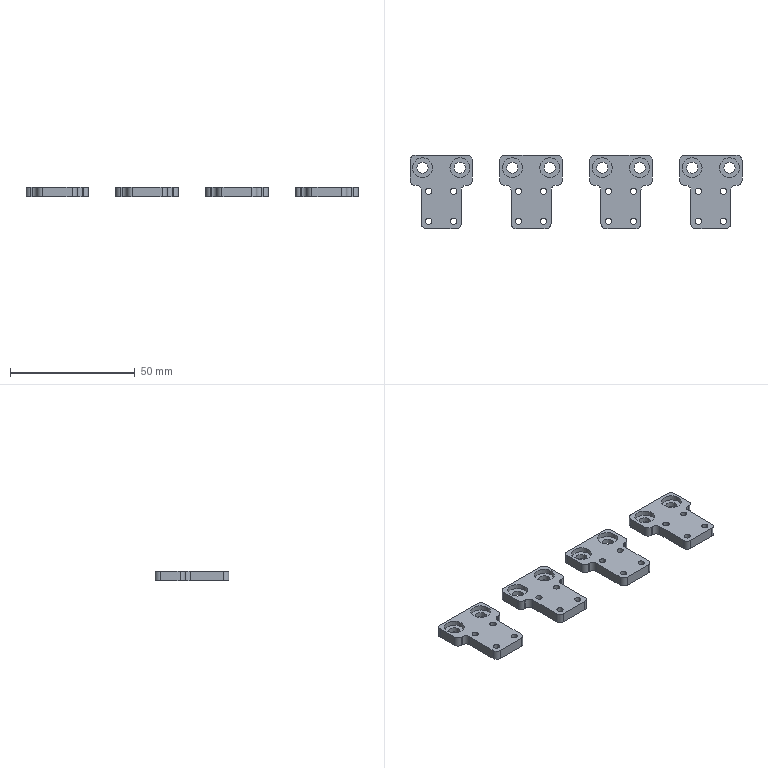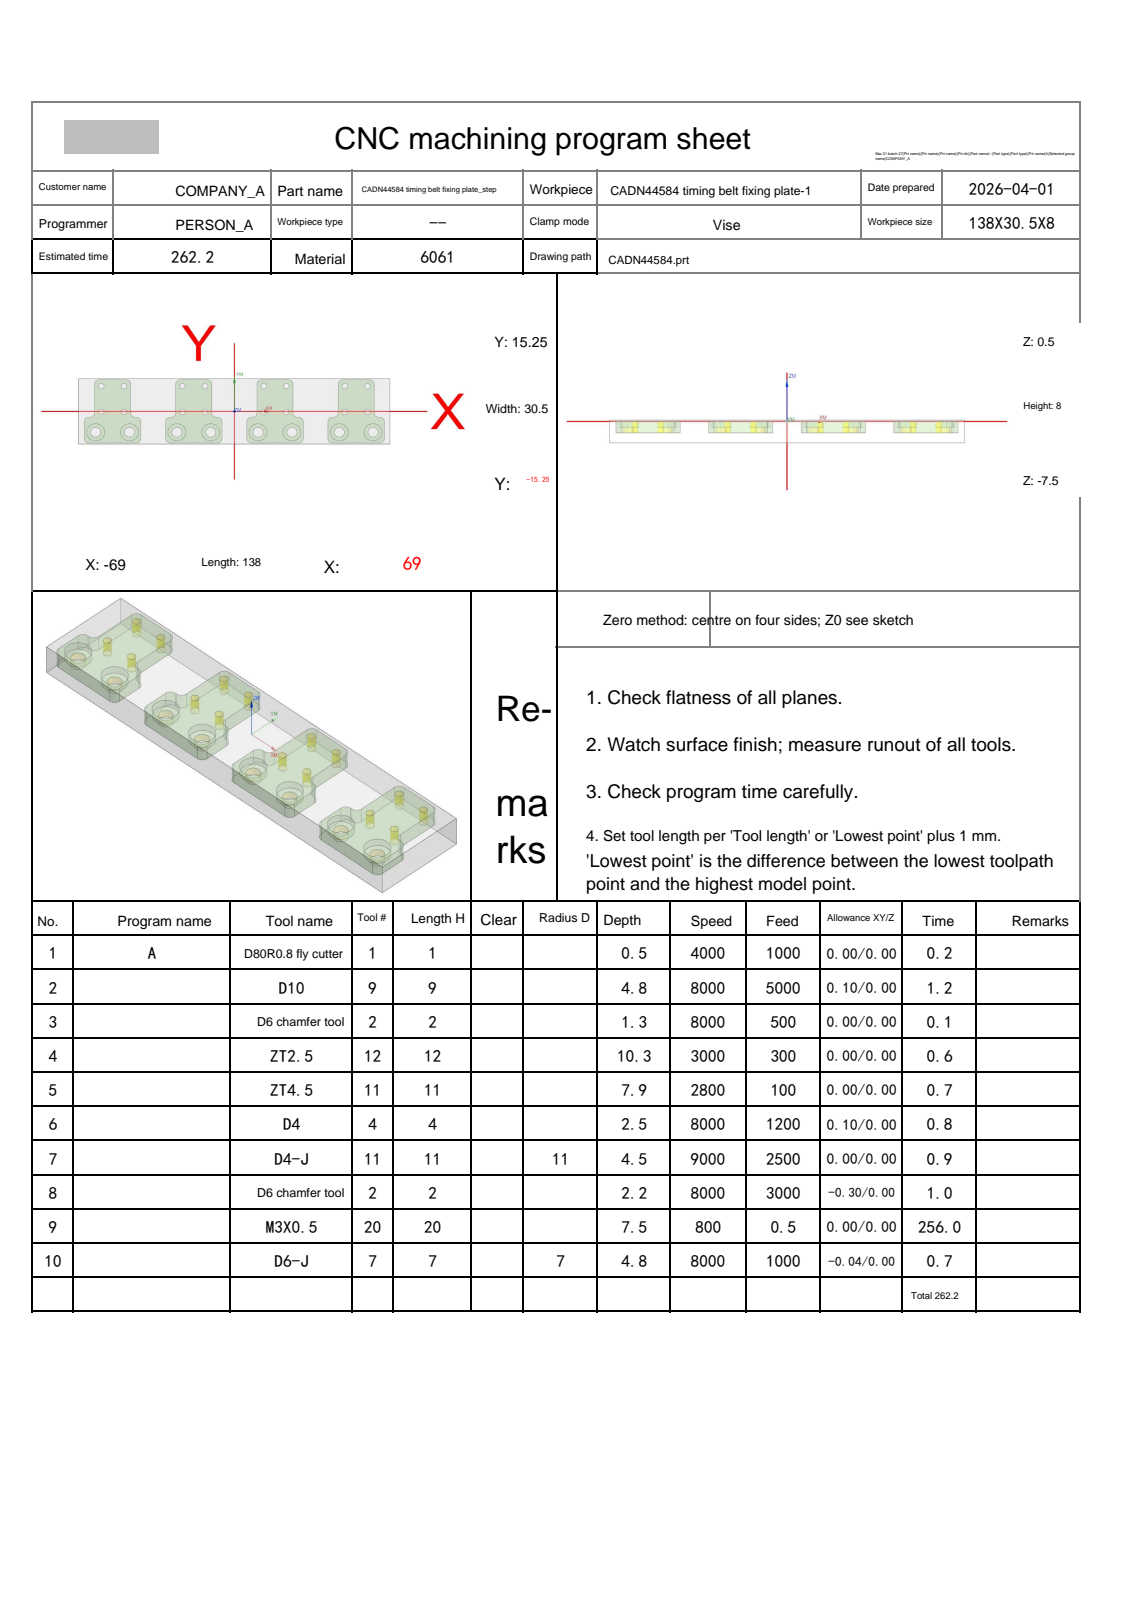NC program | NX | posted by the shop | part box 133 x 29.5 x 4 mm
Lines 4410 to 5056 of 5056:
N8 T02 M06
(D6 chamfer tool  D=6. R=0. H=02 ce=0.00 di=0.00)
G00 G90 G54 X54.25 Y-16.878 M03 S8000
G43 H02 Z20.
M08
Z2.099
G01 Z-1.5 F3000.
G03 X54.33 Y-16.578 I-.52 J.3
X54.03 Y-16.058 I-.6 J0.0
G01 X54. Y-16.05
X43.5
G02 X40.2 Y-12.75 I0.0 J3.3
G01 Y-4.75
G02 X43.5 Y-1.45 I3.3 J0.0
G01 X44.
G03 X44.7 Y-.75 I0.0 J.7
G01 Y12.75
G02 X48. Y16.05 I3.3 J0.0
G01 X60.
G02 X63.3 Y12.75 I0.0 J-3.3
G01 Y-.75
G03 X64. Y-1.45 I.7 J0.0
G01 X64.5
G02 X67.8 Y-4.75 I0.0 J-3.3
G01 Y-12.75
G02 X64.5 Y-16.05 I-3.3 J0.0
G01 X54.
X53.97 Y-16.058
G03 X53.67 Y-16.578 I.3 J-.52
X53.75 Y-16.878 I.6 J0.0
G01 Z2.099
G00 Z20.
X18.25
Z2.099
G01 Z-1.5
G03 X18.33 Y-16.578 I-.52 J.3
X18.03 Y-16.058 I-.6 J0.0
G01 X18. Y-16.05
X7.5
G02 X4.2 Y-12.75 I0.0 J3.3
G01 Y-4.75
G02 X7.5 Y-1.45 I3.3 J0.0
G01 X8.
G03 X8.7 Y-.75 I0.0 J.7
G01 Y12.75
G02 X12. Y16.05 I3.3 J0.0
G01 X24.
G02 X27.3 Y12.75 I0.0 J-3.3
G01 Y-.75
G03 X28. Y-1.45 I.7 J0.0
G01 X28.5
G02 X31.8 Y-4.75 I0.0 J-3.3
G01 Y-12.75
G02 X28.5 Y-16.05 I-3.3 J0.0
G01 X18.
X17.97 Y-16.058
G03 X17.67 Y-16.578 I.3 J-.52
X17.75 Y-16.878 I.6 J0.0
G01 Z2.099
G00 Z20.
X-17.75
Z2.099
G01 Z-1.5
G03 X-17.67 Y-16.578 I-.52 J.3
X-17.97 Y-16.058 I-.6 J0.0
G01 X-18. Y-16.05
X-28.5
G02 X-31.8 Y-12.75 I0.0 J3.3
G01 Y-4.75
G02 X-28.5 Y-1.45 I3.3 J0.0
G01 X-28.
G03 X-27.3 Y-.75 I0.0 J.7
G01 Y12.75
G02 X-24. Y16.05 I3.3 J0.0
G01 X-12.
G02 X-8.7 Y12.75 I0.0 J-3.3
G01 Y-.75
G03 X-8. Y-1.45 I.7 J0.0
G01 X-7.5
G02 X-4.2 Y-4.75 I0.0 J-3.3
G01 Y-12.75
G02 X-7.5 Y-16.05 I-3.3 J0.0
G01 X-18.
X-18.03 Y-16.058
G03 X-18.33 Y-16.578 I.3 J-.52
X-18.25 Y-16.878 I.6 J0.0
G01 Z2.099
G00 Z20.
X-53.75
Z2.099
G01 Z-1.5
G03 X-53.67 Y-16.578 I-.52 J.3
X-53.97 Y-16.058 I-.6 J0.0
G01 X-54. Y-16.05
X-64.5
G02 X-67.8 Y-12.75 I0.0 J3.3
G01 Y-4.75
G02 X-64.5 Y-1.45 I3.3 J0.0
G01 X-64.
G03 X-63.3 Y-.75 I0.0 J.7
G01 Y12.75
G02 X-60. Y16.05 I3.3 J0.0
G01 X-48.
G02 X-44.7 Y12.75 I0.0 J-3.3
G01 Y-.75
G03 X-44. Y-1.45 I.7 J0.0
G01 X-43.5
G02 X-40.2 Y-4.75 I0.0 J-3.3
G01 Y-12.75
G02 X-43.5 Y-16.05 I-3.3 J0.0
G01 X-54.
X-54.03 Y-16.058
G03 X-54.33 Y-16.578 I.3 J-.52
X-54.25 Y-16.878 I.6 J0.0
G01 Z2.099
G00 Z20.
G00 G90 X49. Y-.25 M03 S8000
Z20.
G98 G81 X49. Y-.25 Z-1.75 R3. F500.
X59.
Y11.75
X49.
X23.
Y-.25
X13.
Y11.75
X-13.
Y-.25
X-23.
Y11.75
X-49.
X-59.
Y-.25
X-49.
G80
G00 Z20.
G00 G90 X64.712 Y-9.003 M03 S8000
Z20.
Z2.5
G01 X64.66 Y-8.788 Z2.42 F500.
X64.524 Y-8.422 Z2.278
X64.347 Y-8.075 Z2.136
X64.129 Y-7.751 Z1.994
X63.875 Y-7.455 Z1.852
X63.588 Y-7.191 Z1.71
X63.272 Y-6.962 Z1.568
X63.028 Y-6.822 Z1.465
X62.672 Y-6.662 Z1.323
X62.3 Y-6.545 Z1.181
X61.916 Y-6.473 Z1.039
X61.527 Y-6.447 Z.897
X61.138 Y-6.467 Z.755
X60.753 Y-6.533 Z.613
X60.379 Y-6.643 Z.471
X60.02 Y-6.797 Z.329
X59.682 Y-6.992 Z.187
X59.37 Y-7.226 Z.045
X59.087 Y-7.494 Z-.097
X58.838 Y-7.795 Z-.239
X58.626 Y-8.122 Z-.381
X58.454 Y-8.472 Z-.523
X58.325 Y-8.84 Z-.665
X58.24 Y-9.221 Z-.807
X58.2 Y-9.609 Z-.949
Y-9.75 Z-1.
G03 X61.5 Y-13.05 I3.3 J0.0
X64.8 Y-9.75 I0.0 J3.3
X61.5 Y-6.45 I-3.3 J0.0
X58.2 Y-9.75 I0.0 J-3.3
X58.238 Y-10.248 I3.3 J0.0
G01 Z1.5
G00 Z20.
X49.712 Y-9.003
Z2.5
G01 X49.66 Y-8.788 Z2.42
X49.524 Y-8.422 Z2.278
X49.347 Y-8.075 Z2.136
X49.129 Y-7.751 Z1.994
X48.875 Y-7.455 Z1.852
X48.588 Y-7.191 Z1.71
X48.272 Y-6.962 Z1.568
X48.028 Y-6.822 Z1.465
X47.672 Y-6.662 Z1.323
X47.3 Y-6.545 Z1.181
X46.916 Y-6.473 Z1.039
X46.527 Y-6.447 Z.897
X46.138 Y-6.467 Z.755
X45.753 Y-6.533 Z.613
X45.379 Y-6.643 Z.471
X45.02 Y-6.797 Z.329
X44.682 Y-6.992 Z.187
X44.37 Y-7.226 Z.045
X44.087 Y-7.494 Z-.097
X43.838 Y-7.795 Z-.239
X43.626 Y-8.122 Z-.381
X43.454 Y-8.472 Z-.523
X43.325 Y-8.84 Z-.665
X43.24 Y-9.221 Z-.807
X43.2 Y-9.609 Z-.949
Y-9.75 Z-1.
G03 X46.5 Y-13.05 I3.3 J0.0
X49.8 Y-9.75 I0.0 J3.3
X46.5 Y-6.45 I-3.3 J0.0
X43.2 Y-9.75 I0.0 J-3.3
X43.238 Y-10.248 I3.3 J0.0
G01 Z1.5
G00 Z20.
X28.712 Y-9.003
Z2.5
G01 X28.66 Y-8.788 Z2.42
X28.524 Y-8.422 Z2.278
X28.347 Y-8.075 Z2.136
X28.129 Y-7.751 Z1.994
X27.875 Y-7.455 Z1.852
X27.588 Y-7.191 Z1.71
X27.272 Y-6.962 Z1.568
X27.028 Y-6.822 Z1.465
X26.672 Y-6.662 Z1.323
X26.3 Y-6.545 Z1.181
X25.916 Y-6.473 Z1.039
X25.527 Y-6.447 Z.897
X25.138 Y-6.467 Z.755
X24.753 Y-6.533 Z.613
X24.379 Y-6.643 Z.471
X24.02 Y-6.797 Z.329
X23.682 Y-6.992 Z.187
X23.37 Y-7.226 Z.045
X23.087 Y-7.494 Z-.097
X22.838 Y-7.795 Z-.239
X22.626 Y-8.122 Z-.381
X22.454 Y-8.472 Z-.523
X22.325 Y-8.84 Z-.665
X22.24 Y-9.221 Z-.807
X22.2 Y-9.609 Z-.949
Y-9.75 Z-1.
G03 X25.5 Y-13.05 I3.3 J0.0
X28.8 Y-9.75 I0.0 J3.3
X25.5 Y-6.45 I-3.3 J0.0
X22.2 Y-9.75 I0.0 J-3.3
X22.238 Y-10.248 I3.3 J0.0
G01 Z1.5
G00 Z20.
X13.712 Y-9.003
Z2.5
G01 X13.66 Y-8.788 Z2.42
X13.524 Y-8.422 Z2.278
X13.347 Y-8.075 Z2.136
X13.129 Y-7.751 Z1.994
X12.875 Y-7.455 Z1.852
X12.588 Y-7.191 Z1.71
X12.272 Y-6.962 Z1.568
X12.028 Y-6.822 Z1.465
X11.672 Y-6.662 Z1.323
X11.3 Y-6.545 Z1.181
X10.916 Y-6.473 Z1.039
X10.527 Y-6.447 Z.897
X10.138 Y-6.467 Z.755
X9.753 Y-6.533 Z.613
X9.379 Y-6.643 Z.471
X9.02 Y-6.797 Z.329
X8.682 Y-6.992 Z.187
X8.37 Y-7.226 Z.045
X8.087 Y-7.494 Z-.097
X7.838 Y-7.795 Z-.239
X7.626 Y-8.122 Z-.381
X7.454 Y-8.472 Z-.523
X7.325 Y-8.84 Z-.665
X7.24 Y-9.221 Z-.807
X7.2 Y-9.609 Z-.949
Y-9.75 Z-1.
G03 X10.5 Y-13.05 I3.3 J0.0
X13.8 Y-9.75 I0.0 J3.3
X10.5 Y-6.45 I-3.3 J0.0
X7.2 Y-9.75 I0.0 J-3.3
X7.238 Y-10.248 I3.3 J0.0
G01 Z1.5
G00 Z20.
X-7.288 Y-9.003
Z2.5
G01 X-7.34 Y-8.788 Z2.42
X-7.476 Y-8.422 Z2.278
X-7.653 Y-8.075 Z2.136
X-7.871 Y-7.751 Z1.994
X-8.125 Y-7.455 Z1.852
X-8.412 Y-7.191 Z1.71
X-8.728 Y-6.962 Z1.568
X-8.972 Y-6.822 Z1.465
X-9.328 Y-6.662 Z1.323
X-9.7 Y-6.545 Z1.181
X-10.084 Y-6.473 Z1.039
X-10.473 Y-6.447 Z.897
X-10.862 Y-6.467 Z.755
X-11.247 Y-6.533 Z.613
X-11.621 Y-6.643 Z.471
X-11.98 Y-6.797 Z.329
X-12.318 Y-6.992 Z.187
X-12.63 Y-7.226 Z.045
X-12.913 Y-7.494 Z-.097
X-13.162 Y-7.795 Z-.239
X-13.374 Y-8.122 Z-.381
X-13.546 Y-8.472 Z-.523
X-13.675 Y-8.84 Z-.665
X-13.76 Y-9.221 Z-.807
X-13.8 Y-9.609 Z-.949
Y-9.75 Z-1.
G03 X-10.5 Y-13.05 I3.3 J0.0
X-7.2 Y-9.75 I0.0 J3.3
X-10.5 Y-6.45 I-3.3 J0.0
X-13.8 Y-9.75 I0.0 J-3.3
X-13.762 Y-10.248 I3.3 J0.0
G01 Z1.5
G00 Z20.
X-22.288 Y-9.003
Z2.5
G01 X-22.34 Y-8.788 Z2.42
X-22.476 Y-8.422 Z2.278
X-22.653 Y-8.075 Z2.136
X-22.871 Y-7.751 Z1.994
X-23.125 Y-7.455 Z1.852
X-23.412 Y-7.191 Z1.71
X-23.728 Y-6.962 Z1.568
X-23.972 Y-6.822 Z1.465
X-24.328 Y-6.662 Z1.323
X-24.7 Y-6.545 Z1.181
X-25.084 Y-6.473 Z1.039
X-25.473 Y-6.447 Z.897
X-25.862 Y-6.467 Z.755
X-26.247 Y-6.533 Z.613
X-26.621 Y-6.643 Z.471
X-26.98 Y-6.797 Z.329
X-27.318 Y-6.992 Z.187
X-27.63 Y-7.226 Z.045
X-27.913 Y-7.494 Z-.097
X-28.162 Y-7.795 Z-.239
X-28.374 Y-8.122 Z-.381
X-28.546 Y-8.472 Z-.523
X-28.675 Y-8.84 Z-.665
X-28.76 Y-9.221 Z-.807
X-28.8 Y-9.609 Z-.949
Y-9.75 Z-1.
G03 X-25.5 Y-13.05 I3.3 J0.0
X-22.2 Y-9.75 I0.0 J3.3
X-25.5 Y-6.45 I-3.3 J0.0
X-28.8 Y-9.75 I0.0 J-3.3
X-28.762 Y-10.248 I3.3 J0.0
G01 Z1.5
G00 Z20.
X-43.288 Y-9.003
Z2.5
G01 X-43.34 Y-8.788 Z2.42
X-43.476 Y-8.422 Z2.278
X-43.653 Y-8.075 Z2.136
X-43.871 Y-7.751 Z1.994
X-44.125 Y-7.455 Z1.852
X-44.412 Y-7.191 Z1.71
X-44.728 Y-6.962 Z1.568
X-44.972 Y-6.822 Z1.465
X-45.328 Y-6.662 Z1.323
X-45.7 Y-6.545 Z1.181
X-46.084 Y-6.473 Z1.039
X-46.473 Y-6.447 Z.897
X-46.862 Y-6.467 Z.755
X-47.247 Y-6.533 Z.613
X-47.621 Y-6.643 Z.471
X-47.98 Y-6.797 Z.329
X-48.318 Y-6.992 Z.187
X-48.63 Y-7.226 Z.045
X-48.913 Y-7.494 Z-.097
X-49.162 Y-7.795 Z-.239
X-49.374 Y-8.122 Z-.381
X-49.546 Y-8.472 Z-.523
X-49.675 Y-8.84 Z-.665
X-49.76 Y-9.221 Z-.807
X-49.8 Y-9.609 Z-.949
Y-9.75 Z-1.
G03 X-46.5 Y-13.05 I3.3 J0.0
X-43.2 Y-9.75 I0.0 J3.3
X-46.5 Y-6.45 I-3.3 J0.0
X-49.8 Y-9.75 I0.0 J-3.3
X-49.762 Y-10.248 I3.3 J0.0
G01 Z1.5
G00 Z20.
X-58.288 Y-9.003
Z2.5
G01 X-58.34 Y-8.788 Z2.42
X-58.476 Y-8.422 Z2.278
X-58.653 Y-8.075 Z2.136
X-58.871 Y-7.751 Z1.994
X-59.125 Y-7.455 Z1.852
X-59.412 Y-7.191 Z1.71
X-59.728 Y-6.962 Z1.568
X-59.972 Y-6.822 Z1.465
X-60.328 Y-6.662 Z1.323
X-60.7 Y-6.545 Z1.181
X-61.084 Y-6.473 Z1.039
X-61.473 Y-6.447 Z.897
X-61.862 Y-6.467 Z.755
X-62.247 Y-6.533 Z.613
X-62.621 Y-6.643 Z.471
X-62.98 Y-6.797 Z.329
X-63.318 Y-6.992 Z.187
X-63.63 Y-7.226 Z.045
X-63.913 Y-7.494 Z-.097
X-64.162 Y-7.795 Z-.239
X-64.374 Y-8.122 Z-.381
X-64.546 Y-8.472 Z-.523
X-64.675 Y-8.84 Z-.665
X-64.76 Y-9.221 Z-.807
X-64.8 Y-9.609 Z-.949
Y-9.75 Z-1.
G03 X-61.5 Y-13.05 I3.3 J0.0
X-58.2 Y-9.75 I0.0 J3.3
X-61.5 Y-6.45 I-3.3 J0.0
X-64.8 Y-9.75 I0.0 J-3.3
X-64.762 Y-10.248 I3.3 J0.0
G01 Z1.5
G00 Z20.
G91 G28 Z0.0
M05
M09
G91 G28 Z0.0
M01
N9 T20 M06
(M3X0.5 D=2.5 DR_a=180 H=20)
G00 G90 G54 X49. Y-.25 M03 S800
G43 H20 Z20.
M08
G95
G98 G84 X49. Y-.25 Z-7. R1. F.5 Q5.
X59.
Y11.75
X49.
X23.
Y-.25
X13.
Y11.75
X-13.
Y-.25
X-23.
Y11.75
X-49.
X-59.
Y-.25
X-49.
G80
G94
G00 Z20.
G91 G28 Z0.0
M05
M09
G91 G28 Z0.0
M01
N10 T07 M06
(D6-J  D=6. R=0. H=07 ce=0.00 di=0.00)
G00 G90 G54 X-42.487 Y-18.866 M03 S8000
G43 H07 Z20.
M08
Z-3.8
G01 Z-4.3 F1000.
G41 D07
X-42.503 Y-18.667
G03 X-43.5 Y-17.75 I-.997 J-.083
G01 X-64.5
G02 X-69.5 Y-12.75 I0.0 J5.
G01 Y-4.75
G02 X-65. Y.225 I5. J0.0
G01 Y12.75
G02 X-60. Y17.75 I5. J0.0
G01 X-48.
G02 X-43. Y12.75 I0.0 J-5.
G01 Y.225
G02 X-38.5 Y-4.75 I-.5 J-4.975
G01 Y-12.75
G02 X-43.5 Y-17.75 I-5. J0.0
G01 X-44.
G03 X-45. Y-18.75 I0.0 J-1.
G01 G40 Y-18.95
Z-3.8
G00 Z20.
X-6.487 Y-18.866
Z-3.8
G01 Z-4.3
G41 D07
X-6.503 Y-18.667
G03 X-7.5 Y-17.75 I-.997 J-.083
G01 X-28.5
G02 X-33.5 Y-12.75 I0.0 J5.
G01 Y-4.75
G02 X-29. Y.225 I5. J0.0
G01 Y12.75
G02 X-24. Y17.75 I5. J0.0
G01 X-12.
G02 X-7. Y12.75 I0.0 J-5.
G01 Y.225
G02 X-2.5 Y-4.75 I-.5 J-4.975
G01 Y-12.75
G02 X-7.5 Y-17.75 I-5. J0.0
G01 X-8.
G03 X-9. Y-18.75 I0.0 J-1.
G01 G40 Y-18.95
Z-3.8
G00 Z20.
X29.513 Y-18.866
Z-3.8
G01 Z-4.3
G41 D07
X29.497 Y-18.667
G03 X28.5 Y-17.75 I-.997 J-.083
G01 X7.5
G02 X2.5 Y-12.75 I0.0 J5.
G01 Y-4.75
G02 X7. Y.225 I5. J0.0
G01 Y12.75
G02 X12. Y17.75 I5. J0.0
G01 X24.
G02 X29. Y12.75 I0.0 J-5.
G01 Y.225
G02 X33.5 Y-4.75 I-.5 J-4.975
G01 Y-12.75
G02 X28.5 Y-17.75 I-5. J0.0
G01 X28.
G03 X27. Y-18.75 I0.0 J-1.
G01 G40 Y-18.95
Z-3.8
G00 Z20.
X65.513 Y-18.866
Z-3.8
G01 Z-4.3
G41 D07
X65.497 Y-18.667
G03 X64.5 Y-17.75 I-.997 J-.083
G01 X43.5
G02 X38.5 Y-12.75 I0.0 J5.
G01 Y-4.75
G02 X43. Y.225 I5. J0.0
G01 Y12.75
G02 X48. Y17.75 I5. J0.0
G01 X60.
G02 X65. Y12.75 I0.0 J-5.
G01 Y.225
G02 X69.5 Y-4.75 I-.5 J-4.975
G01 Y-12.75
G02 X64.5 Y-17.75 I-5. J0.0
G01 X64.
G03 X63. Y-18.75 I0.0 J-1.
G01 G40 Y-18.95
Z-3.8
G00 Z20.
G00 G90 X-69.497 Y-16.06 M03 S8000
Z10.5
Z-2.8
G01 Z-4.3 F1000.
G41 D07
X-69.472 Y-15.861
X-69.464 Y-15.806
X-69.465 Y-15.75
Y-1.75
X-69.464 Y-1.694
X-69.472 Y-1.639
G40 X-69.497 Y-1.44
Z-2.8
G00 Z10.5
X-38.503
Z-2.8
G01 Z-4.3
G41 D07
X-38.528 Y-1.639
X-38.536 Y-1.694
X-38.535 Y-1.75
Y-15.75
X-38.536 Y-15.806
X-38.528 Y-15.861
G40 X-38.503 Y-16.06
X-33.497
G41 D07
X-33.472 Y-15.861
X-33.464 Y-15.806
X-33.465 Y-15.75
Y-1.75
X-33.464 Y-1.694
X-33.472 Y-1.639
G40 X-33.497 Y-1.44
Z-2.8
G00 Z10.5
X-2.503
Z-2.8
G01 Z-4.3
G41 D07
X-2.528 Y-1.639
X-2.536 Y-1.694
X-2.535 Y-1.75
Y-15.75
X-2.536 Y-15.806
X-2.528 Y-15.861
G40 X-2.503 Y-16.06
X2.503
G41 D07
X2.528 Y-15.861
X2.536 Y-15.806
X2.535 Y-15.75
Y-1.75
X2.536 Y-1.694
X2.528 Y-1.639
G40 X2.503 Y-1.44
Z-2.8
G00 Z10.5
X33.497
Z-2.8
G01 Z-4.3
G41 D07
X33.472 Y-1.639
X33.464 Y-1.694
X33.465 Y-1.75
Y-15.75
X33.464 Y-15.806
X33.472 Y-15.861
G40 X33.497 Y-16.06
X38.503
G41 D07
X38.528 Y-15.861
X38.536 Y-15.806
X38.535 Y-15.75
Y-1.75
X38.536 Y-1.694
X38.528 Y-1.639
G40 X38.503 Y-1.44
Z-2.8
G00 Z10.5
X69.497
Z-2.8
G01 Z-4.3
G41 D07
X69.472 Y-1.639
X69.464 Y-1.694
X69.465 Y-1.75
Y-15.75
X69.464 Y-15.806
X69.472 Y-15.861
G40 X69.497 Y-16.06
Z-2.8
G00 Z10.5
M05
M09
G91 G28 Z0.0
G91 G28 Y0.0
M30
%